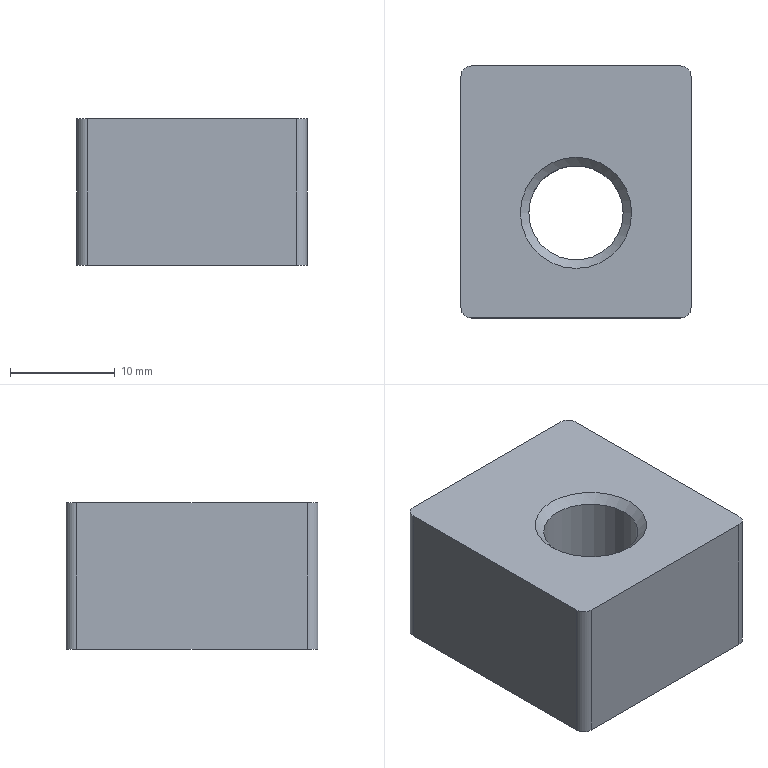CAM job | NX | 3-axis milling, drilling | part box 21.95 x 24 x 14 mm | stock box 24.95 x 27.05 x 14 mm
Tools:
number,name,description,diameter,corner_radius,flute_length,length,flutes
1,D16CU,Milling Tool-5 Parameters,16.0,0.0,50.0,75.0,2
2,D16.,Milling Tool-5 Parameters,16.0,0.0,50.0,75.0,2
3,D8点钻,Chamfer Mill,8.0,0.0,50.0,75.0,2
9,Z9.,Drilling Tool,9.0,0.0,35.0,50.0,2
10,M10-1,Drilling Tool,10.0,0.0,35.0,50.0,4
Operations:
program,operation,operation_type,tool,method,geometry_group,spindle_rpm,surface_speed,feed_per_tooth,feed_cut,feed_plunge,cut_length_mm,path_length_mm,cut_time_min,machine_time_min
G54,ADAPTIVE_MILLING,CavityMilling,D16CU,METHOD,WORKPIECE,2800.0,140.0,0.5357,3000.0,100.0,644.486,768.686,0.1965,0.209
G54,PLANAR_MILL_COPY_1_COPY,PlanarMilling,D16CU,METHOD,WORKPIECE,2500.0,80.0,0.125,400.0,100.0,86.802,186.803,0.217,0.227
G54,PLANAR_MILL,PlanarMilling,D16.,METHOD,WORKPIECE,1600.0,80.0,0.125,400.0,100.0,297.459,426.059,0.7436,0.7565
G54,PLANAR_MILL_COPY_1,PlanarMilling,D16.,METHOD,WORKPIECE,1600.0,80.0,0.125,400.0,100.0,89.949,189.949,0.2249,0.2349
G54,PLANAR_MILL_COPY,PlanarMilling,D8点钻,METHOD,WORKPIECE,4500.0,175.0,0.1714,1200.0,100.0,113.713,219.713,0.0948,0.1054
G54,PLANAR_MILL_COPY_COPY_COPY_COPY,PlanarMilling,D8点钻,METHOD,WORKPIECE,4500.0,175.0,0.1714,1200.0,100.0,18.532,124.532,0.0154,0.026
G54,DRILLING,Operation,D8点钻,METHOD,WORKPIECE,0.0,0.0,0.0,250.0,0.0,3.0,46.0,0.012,0.0163
G54,DRILLING_COPY,Operation,Z9.,METHOD,WORKPIECE,800.0,22.0,0.0625,100.0,0.0,25.0,90.0,0.25,0.2565
G54,DRILLING_COPY_COPY,Operation,M10-1,METHOD,WORKPIECE,200.0,6.0,0.0013,1.0,0.0,19.5,79.0,19.5,19.506
G55,PLANAR_MILL_COPY_1_COPY_COPY,PlanarMilling,D16CU,METHOD,WORKPIECE,2200.0,110.0,0.2727,1200.0,100.0,1736.049,1918.457,1.447,1.465
G55,PLANAR_MILL_COPY_1_COPY_1,PlanarMilling,D16.,METHOD,WORKPIECE,1600.0,80.0,0.125,400.0,100.0,89.949,189.949,0.2249,0.2349
G55,PLANAR_MILL_COPY_COPY,PlanarMilling,D8点钻,METHOD,WORKPIECE,4500.0,175.0,0.1714,1200.0,100.0,113.713,219.713,0.0948,0.1054
G55,PLANAR_MILL_COPY_COPY_COPY,PlanarMilling,D8点钻,METHOD,WORKPIECE,4500.0,175.0,0.1714,1200.0,100.0,18.532,124.532,0.0154,0.026